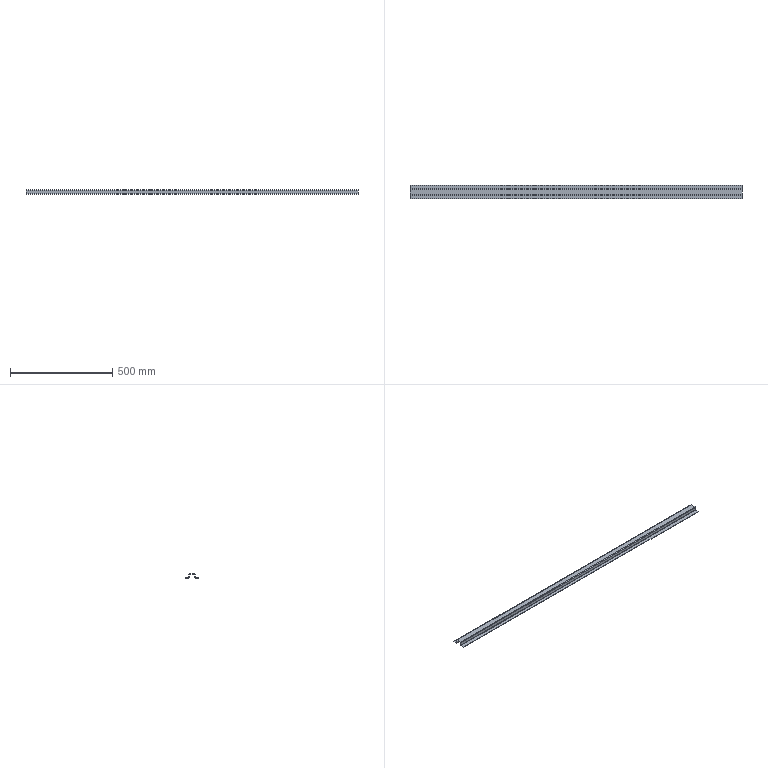Part | SolidWorks | features BaseBody 1 | 1 solid | 38 faces | box 1623 x 66 x 20 mm | volume 319907 mm3 | plane 30 | cylinder 8 | commonest cylinder face diameters 2 x4 6 x4
STEP:
#1=CARTESIAN_POINT('',(-811.4,-33.,-18.));
#2=VERTEX_POINT('',#1);
#3=CARTESIAN_POINT('',(811.4,-33.,-18.));
#4=VERTEX_POINT('',#3);
#5=CARTESIAN_POINT('',(0.,-33.,-18.));
#6=DIRECTION('',(1.,0.,0.));
#7=VECTOR('',#6,1000.);
#8=LINE('',#5,#7);
#9=EDGE_CURVE('',#2,#4,#8,.T.);
#10=ORIENTED_EDGE('',*,*,#9,.F.);
#11=CARTESIAN_POINT('',(-811.4,-33.,-20.));
#12=VERTEX_POINT('',#11);
#13=CARTESIAN_POINT('',(-811.4,-33.,-20.));
#14=DIRECTION('',(0.,0.,1.));
#15=VECTOR('',#14,1000.);
#16=LINE('',#13,#15);
#17=EDGE_CURVE('',#12,#2,#16,.T.);
#18=ORIENTED_EDGE('',*,*,#17,.F.);
#19=CARTESIAN_POINT('',(811.4,-33.,-20.));
#20=VERTEX_POINT('',#19);
#21=CARTESIAN_POINT('',(-811.4,-33.,-20.));
#22=DIRECTION('',(1.,0.,0.));
#23=VECTOR('',#22,1000.);
#24=LINE('',#21,#23);
#25=EDGE_CURVE('',#12,#20,#24,.T.);
#26=ORIENTED_EDGE('',*,*,#25,.T.);
#27=CARTESIAN_POINT('',(811.4,-33.,-20.));
#28=DIRECTION('',(0.,0.,1.));
#29=VECTOR('',#28,1000.);
#30=LINE('',#27,#29);
#31=EDGE_CURVE('',#20,#4,#30,.T.);
#32=ORIENTED_EDGE('',*,*,#31,.T.);
#33=EDGE_LOOP('',(#10,#18,#26,#32));
#34=FACE_OUTER_BOUND('',#33,.T.);
#35=CARTESIAN_POINT('',(-811.4,-33.,-20.));
#36=DIRECTION('',(0.,-1.,0.));
#37=DIRECTION('',(0.,0.,-1.));
#38=AXIS2_PLACEMENT_3D('',#35,#36,#37);
#39=PLANE('',#38);
#40=ADVANCED_FACE('',(#34),#39,.T.);
#41=CARTESIAN_POINT('',(811.4,-16.,-18.));
#42=VERTEX_POINT('',#41);
#43=CARTESIAN_POINT('',(811.4,0.,-18.));
#44=DIRECTION('',(0.,1.,0.));
#45=VECTOR('',#44,1000.);
#46=LINE('',#43,#45);
#47=EDGE_CURVE('',#4,#42,#46,.T.);
#48=ORIENTED_EDGE('',*,*,#47,.T.);
#49=CARTESIAN_POINT('',(-811.4,-16.,-18.));
#50=VERTEX_POINT('',#49);
#51=CARTESIAN_POINT('',(-811.4,-16.,-18.));
#52=DIRECTION('',(1.,0.,0.));
#53=VECTOR('',#52,1000.);
#54=LINE('',#51,#53);
#55=EDGE_CURVE('',#50,#42,#54,.T.);
#56=ORIENTED_EDGE('',*,*,#55,.F.);
#57=CARTESIAN_POINT('',(-811.4,0.,-18.));
#58=DIRECTION('',(0.,-1.,0.));
#59=VECTOR('',#58,1000.);
#60=LINE('',#57,#59);
#61=EDGE_CURVE('',#50,#2,#60,.T.);
#62=ORIENTED_EDGE('',*,*,#61,.T.);
#63=ORIENTED_EDGE('',*,*,#9,.T.);
#64=EDGE_LOOP('',(#48,#56,#62,#63));
#65=FACE_OUTER_BOUND('',#64,.T.);
#66=CARTESIAN_POINT('',(0.,0.,-18.));
#67=DIRECTION('',(0.,0.,1.));
#68=DIRECTION('',(1.,0.,0.));
#69=AXIS2_PLACEMENT_3D('',#66,#67,#68);
#70=PLANE('',#69);
#71=ADVANCED_FACE('',(#65),#70,.T.);
#72=CARTESIAN_POINT('',(811.4,-16.,-20.));
#73=VERTEX_POINT('',#72);
#74=CARTESIAN_POINT('',(-811.4,-16.,-20.));
#75=VERTEX_POINT('',#74);
#76=CARTESIAN_POINT('',(-811.4,-16.,-20.));
#77=DIRECTION('',(-1.,0.,0.));
#78=VECTOR('',#77,1000.);
#79=LINE('',#76,#78);
#80=EDGE_CURVE('',#73,#75,#79,.T.);
#81=ORIENTED_EDGE('',*,*,#80,.F.);
#82=CARTESIAN_POINT('',(811.4,-33.,-20.));
#83=DIRECTION('',(0.,1.,0.));
#84=VECTOR('',#83,1000.);
#85=LINE('',#82,#84);
#86=EDGE_CURVE('',#20,#73,#85,.T.);
#87=ORIENTED_EDGE('',*,*,#86,.F.);
#88=ORIENTED_EDGE('',*,*,#25,.F.);
#89=CARTESIAN_POINT('',(-811.4,-15.,-20.));
#90=DIRECTION('',(0.,-1.,0.));
#91=VECTOR('',#90,1000.);
#92=LINE('',#89,#91);
#93=EDGE_CURVE('',#75,#12,#92,.T.);
#94=ORIENTED_EDGE('',*,*,#93,.F.);
#95=EDGE_LOOP('',(#81,#87,#88,#94));
#96=FACE_OUTER_BOUND('',#95,.T.);
#97=CARTESIAN_POINT('',(0.,0.,-20.));
#98=DIRECTION('',(0.,0.,1.));
#99=DIRECTION('',(1.,0.,0.));
#100=AXIS2_PLACEMENT_3D('',#97,#98,#99);
#101=PLANE('',#100);
#102=ADVANCED_FACE('',(#96),#101,.F.);
#103=ORIENTED_EDGE('',*,*,#86,.T.);
#104=CARTESIAN_POINT('',(811.4,-16.,-18.));
#105=DIRECTION('',(0.,0.,-1.));
#106=VECTOR('',#105,1000.);
#107=LINE('',#104,#106);
#108=EDGE_CURVE('',#42,#73,#107,.T.);
#109=ORIENTED_EDGE('',*,*,#108,.F.);
#110=ORIENTED_EDGE('',*,*,#47,.F.);
#111=ORIENTED_EDGE('',*,*,#31,.F.);
#112=EDGE_LOOP('',(#103,#109,#110,#111));
#113=FACE_OUTER_BOUND('',#112,.T.);
#114=CARTESIAN_POINT('',(811.4,-33.,-20.));
#115=DIRECTION('',(1.,0.,0.));
#116=DIRECTION('',(0.,0.,-1.));
#117=AXIS2_PLACEMENT_3D('',#114,#115,#116);
#118=PLANE('',#117);
#119=ADVANCED_FACE('',(#113),#118,.T.);
#120=ORIENTED_EDGE('',*,*,#61,.F.);
#121=CARTESIAN_POINT('',(-811.4,-16.,-20.));
#122=DIRECTION('',(0.,0.,-1.));
#123=VECTOR('',#122,1000.);
#124=LINE('',#121,#123);
#125=EDGE_CURVE('',#50,#75,#124,.T.);
#126=ORIENTED_EDGE('',*,*,#125,.T.);
#127=ORIENTED_EDGE('',*,*,#93,.T.);
#128=ORIENTED_EDGE('',*,*,#17,.T.);
#129=EDGE_LOOP('',(#120,#126,#127,#128));
#130=FACE_OUTER_BOUND('',#129,.T.);
#131=CARTESIAN_POINT('',(-811.4,-15.,-20.));
#132=DIRECTION('',(-1.,0.,0.));
#133=DIRECTION('',(0.,1.,0.));
#134=AXIS2_PLACEMENT_3D('',#131,#132,#133);
#135=PLANE('',#134);
#136=ADVANCED_FACE('',(#130),#135,.T.);
#137=CARTESIAN_POINT('',(811.4,-15.,-17.));
#138=VERTEX_POINT('',#137);
#139=CARTESIAN_POINT('',(-811.4,-15.,-17.));
#140=VERTEX_POINT('',#139);
#141=CARTESIAN_POINT('',(811.4,-15.,-17.));
#142=DIRECTION('',(-1.,0.,0.));
#143=VECTOR('',#142,1000.);
#144=LINE('',#141,#143);
#145=EDGE_CURVE('',#138,#140,#144,.T.);
#146=ORIENTED_EDGE('',*,*,#145,.T.);
#147=CARTESIAN_POINT('',(-811.4,-16.,-17.));
#148=DIRECTION('',(-1.,0.,0.));
#149=DIRECTION('',(0.,0.,-1.));
#150=AXIS2_PLACEMENT_3D('',#147,#148,#149);
#151=CIRCLE('',#150,1.);
#152=EDGE_CURVE('',#140,#50,#151,.T.);
#153=ORIENTED_EDGE('',*,*,#152,.T.);
#154=ORIENTED_EDGE('',*,*,#55,.T.);
#155=CARTESIAN_POINT('',(811.4,-16.,-17.));
#156=DIRECTION('',(1.,0.,0.));
#157=DIRECTION('',(0.,0.,-1.));
#158=AXIS2_PLACEMENT_3D('',#155,#156,#157);
#159=CIRCLE('',#158,1.);
#160=EDGE_CURVE('',#42,#138,#159,.T.);
#161=ORIENTED_EDGE('',*,*,#160,.T.);
#162=EDGE_LOOP('',(#146,#153,#154,#161));
#163=FACE_OUTER_BOUND('',#162,.T.);
#164=CARTESIAN_POINT('',(811.4,-16.,-17.));
#165=DIRECTION('',(1.,0.,0.));
#166=DIRECTION('',(0.,0.,-1.));
#167=AXIS2_PLACEMENT_3D('',#164,#165,#166);
#168=CYLINDRICAL_SURFACE('',#167,1.);
#169=ADVANCED_FACE('',(#163),#168,.F.);
#170=CARTESIAN_POINT('',(811.4,-13.,-17.));
#171=VERTEX_POINT('',#170);
#172=CARTESIAN_POINT('',(-811.4,-13.,-17.));
#173=VERTEX_POINT('',#172);
#174=CARTESIAN_POINT('',(811.4,-13.,-17.));
#175=DIRECTION('',(-1.,0.,0.));
#176=VECTOR('',#175,1000.);
#177=LINE('',#174,#176);
#178=EDGE_CURVE('',#171,#173,#177,.T.);
#179=ORIENTED_EDGE('',*,*,#178,.F.);
#180=CARTESIAN_POINT('',(811.4,-16.,-17.));
#181=DIRECTION('',(1.,0.,0.));
#182=DIRECTION('',(0.,0.,-1.));
#183=AXIS2_PLACEMENT_3D('',#180,#181,#182);
#184=CIRCLE('',#183,3.);
#185=EDGE_CURVE('',#73,#171,#184,.T.);
#186=ORIENTED_EDGE('',*,*,#185,.F.);
#187=ORIENTED_EDGE('',*,*,#80,.T.);
#188=CARTESIAN_POINT('',(-811.4,-16.,-17.));
#189=DIRECTION('',(-1.,0.,0.));
#190=DIRECTION('',(0.,0.,-1.));
#191=AXIS2_PLACEMENT_3D('',#188,#189,#190);
#192=CIRCLE('',#191,3.);
#193=EDGE_CURVE('',#173,#75,#192,.T.);
#194=ORIENTED_EDGE('',*,*,#193,.F.);
#195=EDGE_LOOP('',(#179,#186,#187,#194));
#196=FACE_OUTER_BOUND('',#195,.T.);
#197=CARTESIAN_POINT('',(811.4,-16.,-17.));
#198=DIRECTION('',(1.,0.,0.));
#199=DIRECTION('',(0.,0.,-1.));
#200=AXIS2_PLACEMENT_3D('',#197,#198,#199);
#201=CYLINDRICAL_SURFACE('',#200,3.);
#202=ADVANCED_FACE('',(#196),#201,.T.);
#203=ORIENTED_EDGE('',*,*,#160,.F.);
#204=ORIENTED_EDGE('',*,*,#108,.T.);
#205=ORIENTED_EDGE('',*,*,#185,.T.);
#206=CARTESIAN_POINT('',(811.4,-15.,-17.));
#207=DIRECTION('',(0.,1.,0.));
#208=VECTOR('',#207,1000.);
#209=LINE('',#206,#208);
#210=EDGE_CURVE('',#138,#171,#209,.T.);
#211=ORIENTED_EDGE('',*,*,#210,.F.);
#212=EDGE_LOOP('',(#203,#204,#205,#211));
#213=FACE_OUTER_BOUND('',#212,.T.);
#214=CARTESIAN_POINT('',(811.4,-16.,-17.));
#215=DIRECTION('',(-1.,0.,0.));
#216=DIRECTION('',(0.,0.,1.));
#217=AXIS2_PLACEMENT_3D('',#214,#215,#216);
#218=PLANE('',#217);
#219=ADVANCED_FACE('',(#213),#218,.F.);
#220=ORIENTED_EDGE('',*,*,#125,.F.);
#221=ORIENTED_EDGE('',*,*,#152,.F.);
#222=CARTESIAN_POINT('',(-811.4,-15.,-17.));
#223=DIRECTION('',(0.,1.,0.));
#224=VECTOR('',#223,1000.);
#225=LINE('',#222,#224);
#226=EDGE_CURVE('',#140,#173,#225,.T.);
#227=ORIENTED_EDGE('',*,*,#226,.T.);
#228=ORIENTED_EDGE('',*,*,#193,.T.);
#229=EDGE_LOOP('',(#220,#221,#227,#228));
#230=FACE_OUTER_BOUND('',#229,.T.);
#231=CARTESIAN_POINT('',(-811.4,-16.,-17.));
#232=DIRECTION('',(-1.,0.,0.));
#233=DIRECTION('',(0.,0.,1.));
#234=AXIS2_PLACEMENT_3D('',#231,#232,#233);
#235=PLANE('',#234);
#236=ADVANCED_FACE('',(#230),#235,.T.);
#237=CARTESIAN_POINT('',(811.4,33.,-18.));
#238=VERTEX_POINT('',#237);
#239=CARTESIAN_POINT('',(-811.4,33.,-18.));
#240=VERTEX_POINT('',#239);
#241=CARTESIAN_POINT('',(0.,33.,-18.));
#242=DIRECTION('',(-1.,0.,0.));
#243=VECTOR('',#242,1000.);
#244=LINE('',#241,#243);
#245=EDGE_CURVE('',#238,#240,#244,.T.);
#246=ORIENTED_EDGE('',*,*,#245,.F.);
#247=CARTESIAN_POINT('',(811.4,33.,-20.));
#248=VERTEX_POINT('',#247);
#249=CARTESIAN_POINT('',(811.4,33.,-20.));
#250=DIRECTION('',(0.,0.,1.));
#251=VECTOR('',#250,1000.);
#252=LINE('',#249,#251);
#253=EDGE_CURVE('',#248,#238,#252,.T.);
#254=ORIENTED_EDGE('',*,*,#253,.F.);
#255=CARTESIAN_POINT('',(-811.4,33.,-20.));
#256=VERTEX_POINT('',#255);
#257=CARTESIAN_POINT('',(-811.4,33.,-20.));
#258=DIRECTION('',(-1.,0.,0.));
#259=VECTOR('',#258,1000.);
#260=LINE('',#257,#259);
#261=EDGE_CURVE('',#248,#256,#260,.T.);
#262=ORIENTED_EDGE('',*,*,#261,.T.);
#263=CARTESIAN_POINT('',(-811.4,33.,-20.));
#264=DIRECTION('',(0.,0.,1.));
#265=VECTOR('',#264,1000.);
#266=LINE('',#263,#265);
#267=EDGE_CURVE('',#256,#240,#266,.T.);
#268=ORIENTED_EDGE('',*,*,#267,.T.);
#269=EDGE_LOOP('',(#246,#254,#262,#268));
#270=FACE_OUTER_BOUND('',#269,.T.);
#271=CARTESIAN_POINT('',(-811.4,33.,-20.));
#272=DIRECTION('',(0.,1.,0.));
#273=DIRECTION('',(1.,0.,0.));
#274=AXIS2_PLACEMENT_3D('',#271,#272,#273);
#275=PLANE('',#274);
#276=ADVANCED_FACE('',(#270),#275,.T.);
#277=CARTESIAN_POINT('',(811.4,16.,-18.));
#278=VERTEX_POINT('',#277);
#279=CARTESIAN_POINT('',(-811.4,16.,-18.));
#280=VERTEX_POINT('',#279);
#281=CARTESIAN_POINT('',(811.4,16.,-18.));
#282=DIRECTION('',(-1.,0.,0.));
#283=VECTOR('',#282,1000.);
#284=LINE('',#281,#283);
#285=EDGE_CURVE('',#278,#280,#284,.T.);
#286=ORIENTED_EDGE('',*,*,#285,.F.);
#287=CARTESIAN_POINT('',(811.4,0.,-18.));
#288=DIRECTION('',(0.,1.,0.));
#289=VECTOR('',#288,1000.);
#290=LINE('',#287,#289);
#291=EDGE_CURVE('',#278,#238,#290,.T.);
#292=ORIENTED_EDGE('',*,*,#291,.T.);
#293=ORIENTED_EDGE('',*,*,#245,.T.);
#294=CARTESIAN_POINT('',(-811.4,0.,-18.));
#295=DIRECTION('',(0.,-1.,0.));
#296=VECTOR('',#295,1000.);
#297=LINE('',#294,#296);
#298=EDGE_CURVE('',#240,#280,#297,.T.);
#299=ORIENTED_EDGE('',*,*,#298,.T.);
#300=EDGE_LOOP('',(#286,#292,#293,#299));
#301=FACE_OUTER_BOUND('',#300,.T.);
#302=CARTESIAN_POINT('',(0.,0.,-18.));
#303=DIRECTION('',(0.,0.,-1.));
#304=DIRECTION('',(0.,-1.,0.));
#305=AXIS2_PLACEMENT_3D('',#302,#303,#304);
#306=PLANE('',#305);
#307=ADVANCED_FACE('',(#301),#306,.F.);
#308=CARTESIAN_POINT('',(811.4,16.,-20.));
#309=VERTEX_POINT('',#308);
#310=CARTESIAN_POINT('',(811.4,33.,-20.));
#311=DIRECTION('',(0.,1.,0.));
#312=VECTOR('',#311,1000.);
#313=LINE('',#310,#312);
#314=EDGE_CURVE('',#309,#248,#313,.T.);
#315=ORIENTED_EDGE('',*,*,#314,.F.);
#316=CARTESIAN_POINT('',(-811.4,16.,-20.));
#317=VERTEX_POINT('',#316);
#318=CARTESIAN_POINT('',(0.,16.,-20.));
#319=DIRECTION('',(-1.,0.,0.));
#320=VECTOR('',#319,1000.);
#321=LINE('',#318,#320);
#322=EDGE_CURVE('',#309,#317,#321,.T.);
#323=ORIENTED_EDGE('',*,*,#322,.T.);
#324=CARTESIAN_POINT('',(-811.4,33.,-20.));
#325=DIRECTION('',(0.,-1.,0.));
#326=VECTOR('',#325,1000.);
#327=LINE('',#324,#326);
#328=EDGE_CURVE('',#256,#317,#327,.T.);
#329=ORIENTED_EDGE('',*,*,#328,.F.);
#330=ORIENTED_EDGE('',*,*,#261,.F.);
#331=EDGE_LOOP('',(#315,#323,#329,#330));
#332=FACE_OUTER_BOUND('',#331,.T.);
#333=CARTESIAN_POINT('',(0.,0.,-20.));
#334=DIRECTION('',(0.,0.,-1.));
#335=DIRECTION('',(0.,-1.,0.));
#336=AXIS2_PLACEMENT_3D('',#333,#334,#335);
#337=PLANE('',#336);
#338=ADVANCED_FACE('',(#332),#337,.T.);
#339=ORIENTED_EDGE('',*,*,#328,.T.);
#340=CARTESIAN_POINT('',(-811.4,16.,-18.));
#341=DIRECTION('',(0.,0.,-1.));
#342=VECTOR('',#341,1000.);
#343=LINE('',#340,#342);
#344=EDGE_CURVE('',#280,#317,#343,.T.);
#345=ORIENTED_EDGE('',*,*,#344,.F.);
#346=ORIENTED_EDGE('',*,*,#298,.F.);
#347=ORIENTED_EDGE('',*,*,#267,.F.);
#348=EDGE_LOOP('',(#339,#345,#346,#347));
#349=FACE_OUTER_BOUND('',#348,.T.);
#350=CARTESIAN_POINT('',(-811.4,33.,-20.));
#351=DIRECTION('',(-1.,0.,0.));
#352=DIRECTION('',(0.,0.,1.));
#353=AXIS2_PLACEMENT_3D('',#350,#351,#352);
#354=PLANE('',#353);
#355=ADVANCED_FACE('',(#349),#354,.T.);
#356=ORIENTED_EDGE('',*,*,#291,.F.);
#357=CARTESIAN_POINT('',(811.4,16.,-20.));
#358=DIRECTION('',(0.,0.,-1.));
#359=VECTOR('',#358,1000.);
#360=LINE('',#357,#359);
#361=EDGE_CURVE('',#278,#309,#360,.T.);
#362=ORIENTED_EDGE('',*,*,#361,.T.);
#363=ORIENTED_EDGE('',*,*,#314,.T.);
#364=ORIENTED_EDGE('',*,*,#253,.T.);
#365=EDGE_LOOP('',(#356,#362,#363,#364));
#366=FACE_OUTER_BOUND('',#365,.T.);
#367=CARTESIAN_POINT('',(811.4,33.,-20.));
#368=DIRECTION('',(1.,0.,0.));
#369=DIRECTION('',(0.,1.,0.));
#370=AXIS2_PLACEMENT_3D('',#367,#368,#369);
#371=PLANE('',#370);
#372=ADVANCED_FACE('',(#366),#371,.T.);
#373=CARTESIAN_POINT('',(-811.4,15.,-17.));
#374=VERTEX_POINT('',#373);
#375=CARTESIAN_POINT('',(811.4,15.,-17.));
#376=VERTEX_POINT('',#375);
#377=CARTESIAN_POINT('',(-811.4,15.,-17.));
#378=DIRECTION('',(1.,0.,0.));
#379=VECTOR('',#378,1000.);
#380=LINE('',#377,#379);
#381=EDGE_CURVE('',#374,#376,#380,.T.);
#382=ORIENTED_EDGE('',*,*,#381,.T.);
#383=CARTESIAN_POINT('',(811.4,16.,-17.));
#384=DIRECTION('',(1.,0.,0.));
#385=DIRECTION('',(0.,0.,1.));
#386=AXIS2_PLACEMENT_3D('',#383,#384,#385);
#387=CIRCLE('',#386,1.);
#388=EDGE_CURVE('',#376,#278,#387,.T.);
#389=ORIENTED_EDGE('',*,*,#388,.T.);
#390=ORIENTED_EDGE('',*,*,#285,.T.);
#391=CARTESIAN_POINT('',(-811.4,16.,-17.));
#392=DIRECTION('',(-1.,0.,0.));
#393=DIRECTION('',(0.,0.,1.));
#394=AXIS2_PLACEMENT_3D('',#391,#392,#393);
#395=CIRCLE('',#394,1.);
#396=EDGE_CURVE('',#280,#374,#395,.T.);
#397=ORIENTED_EDGE('',*,*,#396,.T.);
#398=EDGE_LOOP('',(#382,#389,#390,#397));
#399=FACE_OUTER_BOUND('',#398,.T.);
#400=CARTESIAN_POINT('',(-811.4,16.,-17.));
#401=DIRECTION('',(-1.,0.,0.));
#402=DIRECTION('',(0.,0.,-1.));
#403=AXIS2_PLACEMENT_3D('',#400,#401,#402);
#404=CYLINDRICAL_SURFACE('',#403,1.);
#405=ADVANCED_FACE('',(#399),#404,.F.);
#406=CARTESIAN_POINT('',(-811.4,13.,-17.));
#407=VERTEX_POINT('',#406);
#408=CARTESIAN_POINT('',(811.4,13.,-17.));
#409=VERTEX_POINT('',#408);
#410=CARTESIAN_POINT('',(-811.4,13.,-17.));
#411=DIRECTION('',(1.,0.,0.));
#412=VECTOR('',#411,1000.);
#413=LINE('',#410,#412);
#414=EDGE_CURVE('',#407,#409,#413,.T.);
#415=ORIENTED_EDGE('',*,*,#414,.F.);
#416=CARTESIAN_POINT('',(-811.4,16.,-17.));
#417=DIRECTION('',(-1.,0.,0.));
#418=DIRECTION('',(0.,0.,1.));
#419=AXIS2_PLACEMENT_3D('',#416,#417,#418);
#420=CIRCLE('',#419,3.);
#421=EDGE_CURVE('',#317,#407,#420,.T.);
#422=ORIENTED_EDGE('',*,*,#421,.F.);
#423=ORIENTED_EDGE('',*,*,#322,.F.);
#424=CARTESIAN_POINT('',(811.4,16.,-17.));
#425=DIRECTION('',(1.,0.,0.));
#426=DIRECTION('',(0.,0.,1.));
#427=AXIS2_PLACEMENT_3D('',#424,#425,#426);
#428=CIRCLE('',#427,3.);
#429=EDGE_CURVE('',#409,#309,#428,.T.);
#430=ORIENTED_EDGE('',*,*,#429,.F.);
#431=EDGE_LOOP('',(#415,#422,#423,#430));
#432=FACE_OUTER_BOUND('',#431,.T.);
#433=CARTESIAN_POINT('',(-811.4,16.,-17.));
#434=DIRECTION('',(-1.,0.,0.));
#435=DIRECTION('',(0.,0.,-1.));
#436=AXIS2_PLACEMENT_3D('',#433,#434,#435);
#437=CYLINDRICAL_SURFACE('',#436,3.);
#438=ADVANCED_FACE('',(#432),#437,.T.);
#439=ORIENTED_EDGE('',*,*,#396,.F.);
#440=ORIENTED_EDGE('',*,*,#344,.T.);
#441=ORIENTED_EDGE('',*,*,#421,.T.);
#442=CARTESIAN_POINT('',(-811.4,15.,-17.));
#443=DIRECTION('',(0.,-1.,0.));
#444=VECTOR('',#443,1000.);
#445=LINE('',#442,#444);
#446=EDGE_CURVE('',#374,#407,#445,.T.);
#447=ORIENTED_EDGE('',*,*,#446,.F.);
#448=EDGE_LOOP('',(#439,#440,#441,#447));
#449=FACE_OUTER_BOUND('',#448,.T.);
#450=CARTESIAN_POINT('',(-811.4,16.,-17.));
#451=DIRECTION('',(1.,0.,0.));
#452=DIRECTION('',(0.,1.,0.));
#453=AXIS2_PLACEMENT_3D('',#450,#451,#452);
#454=PLANE('',#453);
#455=ADVANCED_FACE('',(#449),#454,.F.);
#456=ORIENTED_EDGE('',*,*,#361,.F.);
#457=ORIENTED_EDGE('',*,*,#388,.F.);
#458=CARTESIAN_POINT('',(811.4,15.,-17.));
#459=DIRECTION('',(0.,-1.,0.));
#460=VECTOR('',#459,1000.);
#461=LINE('',#458,#460);
#462=EDGE_CURVE('',#376,#409,#461,.T.);
#463=ORIENTED_EDGE('',*,*,#462,.T.);
#464=ORIENTED_EDGE('',*,*,#429,.T.);
#465=EDGE_LOOP('',(#456,#457,#463,#464));
#466=FACE_OUTER_BOUND('',#465,.T.);
#467=CARTESIAN_POINT('',(811.4,16.,-17.));
#468=DIRECTION('',(1.,0.,0.));
#469=DIRECTION('',(0.,1.,0.));
#470=AXIS2_PLACEMENT_3D('',#467,#468,#469);
#471=PLANE('',#470);
#472=ADVANCED_FACE('',(#466),#471,.T.);
#473=ORIENTED_EDGE('',*,*,#226,.F.);
#474=CARTESIAN_POINT('',(-811.4,-15.,-3.));
#475=VERTEX_POINT('',#474);
#476=CARTESIAN_POINT('',(-811.4,-15.,-20.));
#477=DIRECTION('',(0.,0.,1.));
#478=VECTOR('',#477,1000.);
#479=LINE('',#476,#478);
#480=EDGE_CURVE('',#140,#475,#479,.T.);
#481=ORIENTED_EDGE('',*,*,#480,.T.);
#482=CARTESIAN_POINT('',(-811.4,-13.,-3.));
#483=VERTEX_POINT('',#482);
#484=CARTESIAN_POINT('',(-811.4,-13.,-3.));
#485=DIRECTION('',(0.,-1.,0.));
#486=VECTOR('',#485,1000.);
#487=LINE('',#484,#486);
#488=EDGE_CURVE('',#483,#475,#487,.T.);
#489=ORIENTED_EDGE('',*,*,#488,.F.);
#490=CARTESIAN_POINT('',(-811.4,-13.,0.));
#491=DIRECTION('',(0.,0.,1.));
#492=VECTOR('',#491,1000.);
#493=LINE('',#490,#492);
#494=EDGE_CURVE('',#173,#483,#493,.T.);
#495=ORIENTED_EDGE('',*,*,#494,.F.);
#496=EDGE_LOOP('',(#473,#481,#489,#495));
#497=FACE_OUTER_BOUND('',#496,.T.);
#498=CARTESIAN_POINT('',(-811.4,-15.,-20.));
#499=DIRECTION('',(-1.,0.,0.));
#500=DIRECTION('',(0.,0.,1.));
#501=AXIS2_PLACEMENT_3D('',#498,#499,#500);
#502=PLANE('',#501);
#503=ADVANCED_FACE('',(#497),#502,.T.);
#504=CARTESIAN_POINT('',(-811.4,-12.,-2.));
#505=VERTEX_POINT('',#504);
#506=CARTESIAN_POINT('',(811.4,-12.,-2.));
#507=VERTEX_POINT('',#506);
#508=CARTESIAN_POINT('',(-811.4,-12.,-2.));
#509=DIRECTION('',(1.,0.,0.));
#510=VECTOR('',#509,1000.);
#511=LINE('',#508,#510);
#512=EDGE_CURVE('',#505,#507,#511,.T.);
#513=ORIENTED_EDGE('',*,*,#512,.T.);
#514=CARTESIAN_POINT('',(811.4,-13.,-3.));
#515=VERTEX_POINT('',#514);
#516=CARTESIAN_POINT('',(811.4,-12.,-3.));
#517=DIRECTION('',(1.,0.,0.));
#518=DIRECTION('',(0.,0.,1.));
#519=AXIS2_PLACEMENT_3D('',#516,#517,#518);
#520=CIRCLE('',#519,1.);
#521=EDGE_CURVE('',#507,#515,#520,.T.);
#522=ORIENTED_EDGE('',*,*,#521,.T.);
#523=CARTESIAN_POINT('',(811.4,-13.,-3.));
#524=DIRECTION('',(-1.,0.,0.));
#525=VECTOR('',#524,1000.);
#526=LINE('',#523,#525);
#527=EDGE_CURVE('',#515,#483,#526,.T.);
#528=ORIENTED_EDGE('',*,*,#527,.T.);
#529=CARTESIAN_POINT('',(-811.4,-12.,-3.));
#530=DIRECTION('',(-1.,0.,0.));
#531=DIRECTION('',(0.,0.,1.));
#532=AXIS2_PLACEMENT_3D('',#529,#530,#531);
#533=CIRCLE('',#532,1.);
#534=EDGE_CURVE('',#483,#505,#533,.T.);
#535=ORIENTED_EDGE('',*,*,#534,.T.);
#536=EDGE_LOOP('',(#513,#522,#528,#535));
#537=FACE_OUTER_BOUND('',#536,.T.);
#538=CARTESIAN_POINT('',(-811.4,-12.,-3.));
#539=DIRECTION('',(-1.,0.,0.));
#540=DIRECTION('',(0.,-1.,0.));
#541=AXIS2_PLACEMENT_3D('',#538,#539,#540);
#542=CYLINDRICAL_SURFACE('',#541,1.);
#543=ADVANCED_FACE('',(#537),#542,.F.);
#544=CARTESIAN_POINT('',(-811.4,-12.,0.));
#545=VERTEX_POINT('',#544);
#546=CARTESIAN_POINT('',(811.4,-12.,0.));
#547=VERTEX_POINT('',#546);
#548=CARTESIAN_POINT('',(-811.4,-12.,0.));
#549=DIRECTION('',(1.,0.,0.));
#550=VECTOR('',#549,1000.);
#551=LINE('',#548,#550);
#552=EDGE_CURVE('',#545,#547,#551,.T.);
#553=ORIENTED_EDGE('',*,*,#552,.F.);
#554=CARTESIAN_POINT('',(-811.4,-12.,-3.));
#555=DIRECTION('',(-1.,0.,0.));
#556=DIRECTION('',(0.,0.,1.));
#557=AXIS2_PLACEMENT_3D('',#554,#555,#556);
#558=CIRCLE('',#557,3.);
#559=EDGE_CURVE('',#475,#545,#558,.T.);
#560=ORIENTED_EDGE('',*,*,#559,.F.);
#561=CARTESIAN_POINT('',(811.4,-15.,-3.));
#562=VERTEX_POINT('',#561);
#563=CARTESIAN_POINT('',(811.4,-15.,-3.));
#564=DIRECTION('',(1.,0.,0.));
#565=VECTOR('',#564,1000.);
#566=LINE('',#563,#565);
#567=EDGE_CURVE('',#475,#562,#566,.T.);
#568=ORIENTED_EDGE('',*,*,#567,.T.);
#569=CARTESIAN_POINT('',(811.4,-12.,-3.));
#570=DIRECTION('',(1.,0.,0.));
#571=DIRECTION('',(0.,0.,1.));
#572=AXIS2_PLACEMENT_3D('',#569,#570,#571);
#573=CIRCLE('',#572,3.);
#574=EDGE_CURVE('',#547,#562,#573,.T.);
#575=ORIENTED_EDGE('',*,*,#574,.F.);
#576=EDGE_LOOP('',(#553,#560,#568,#575));
#577=FACE_OUTER_BOUND('',#576,.T.);
#578=CARTESIAN_POINT('',(-811.4,-12.,-3.));
#579=DIRECTION('',(-1.,0.,0.));
#580=DIRECTION('',(0.,-1.,0.));
#581=AXIS2_PLACEMENT_3D('',#578,#579,#580);
#582=CYLINDRICAL_SURFACE('',#581,3.);
#583=ADVANCED_FACE('',(#577),#582,.T.);
#584=ORIENTED_EDGE('',*,*,#534,.F.);
#585=ORIENTED_EDGE('',*,*,#488,.T.);
#586=ORIENTED_EDGE('',*,*,#559,.T.);
#587=CARTESIAN_POINT('',(-811.4,-12.,-2.));
#588=DIRECTION('',(0.,0.,1.));
#589=VECTOR('',#588,1000.);
#590=LINE('',#587,#589);
#591=EDGE_CURVE('',#505,#545,#590,.T.);
#592=ORIENTED_EDGE('',*,*,#591,.F.);
#593=EDGE_LOOP('',(#584,#585,#586,#592));
#594=FACE_OUTER_BOUND('',#593,.T.);
#595=CARTESIAN_POINT('',(-811.4,-12.,-3.));
#596=DIRECTION('',(1.,0.,0.));
#597=DIRECTION('',(0.,1.,0.));
#598=AXIS2_PLACEMENT_3D('',#595,#596,#597);
#599=PLANE('',#598);
#600=ADVANCED_FACE('',(#594),#599,.F.);
#601=CARTESIAN_POINT('',(811.4,-15.,-3.));
#602=DIRECTION('',(0.,-1.,0.));
#603=VECTOR('',#602,1000.);
#604=LINE('',#601,#603);
#605=EDGE_CURVE('',#515,#562,#604,.T.);
#606=ORIENTED_EDGE('',*,*,#605,.F.);
#607=ORIENTED_EDGE('',*,*,#521,.F.);
#608=CARTESIAN_POINT('',(811.4,-12.,-2.));
#609=DIRECTION('',(0.,0.,1.));
#610=VECTOR('',#609,1000.);
#611=LINE('',#608,#610);
#612=EDGE_CURVE('',#507,#547,#611,.T.);
#613=ORIENTED_EDGE('',*,*,#612,.T.);
#614=ORIENTED_EDGE('',*,*,#574,.T.);
#615=EDGE_LOOP('',(#606,#607,#613,#614));
#616=FACE_OUTER_BOUND('',#615,.T.);
#617=CARTESIAN_POINT('',(811.4,-12.,-3.));
#618=DIRECTION('',(1.,0.,0.));
#619=DIRECTION('',(0.,1.,0.));
#620=AXIS2_PLACEMENT_3D('',#617,#618,#619);
#621=PLANE('',#620);
#622=ADVANCED_FACE('',(#616),#621,.T.);
#623=ORIENTED_EDGE('',*,*,#462,.F.);
#624=CARTESIAN_POINT('',(811.4,15.,-3.));
#625=VERTEX_POINT('',#624);
#626=CARTESIAN_POINT('',(811.4,15.,-2.));
#627=DIRECTION('',(0.,0.,1.));
#628=VECTOR('',#627,1000.);
#629=LINE('',#626,#628);
#630=EDGE_CURVE('',#376,#625,#629,.T.);
#631=ORIENTED_EDGE('',*,*,#630,.T.);
#632=CARTESIAN_POINT('',(811.4,13.,-3.));
#633=VERTEX_POINT('',#632);
#634=CARTESIAN_POINT('',(811.4,13.,-3.));
#635=DIRECTION('',(0.,1.,0.));
#636=VECTOR('',#635,1000.);
#637=LINE('',#634,#636);
#638=EDGE_CURVE('',#633,#625,#637,.T.);
#639=ORIENTED_EDGE('',*,*,#638,.F.);
#640=CARTESIAN_POINT('',(811.4,13.,0.));
#641=DIRECTION('',(0.,0.,1.));
#642=VECTOR('',#641,1000.);
#643=LINE('',#640,#642);
#644=EDGE_CURVE('',#409,#633,#643,.T.);
#645=ORIENTED_EDGE('',*,*,#644,.F.);
#646=EDGE_LOOP('',(#623,#631,#639,#645));
#647=FACE_OUTER_BOUND('',#646,.T.);
#648=CARTESIAN_POINT('',(811.4,15.,-2.));
#649=DIRECTION('',(1.,0.,0.));
#650=DIRECTION('',(0.,1.,0.));
#651=AXIS2_PLACEMENT_3D('',#648,#649,#650);
#652=PLANE('',#651);
#653=ADVANCED_FACE('',(#647),#652,.T.);
#654=CARTESIAN_POINT('',(811.4,12.,-2.));
#655=VERTEX_POINT('',#654);
#656=CARTESIAN_POINT('',(-811.4,12.,-2.));
#657=VERTEX_POINT('',#656);
#658=CARTESIAN_POINT('',(811.4,12.,-2.));
#659=DIRECTION('',(-1.,0.,0.));
#660=VECTOR('',#659,1000.);
#661=LINE('',#658,#660);
#662=EDGE_CURVE('',#655,#657,#661,.T.);
#663=ORIENTED_EDGE('',*,*,#662,.T.);
#664=CARTESIAN_POINT('',(-811.4,13.,-3.));
#665=VERTEX_POINT('',#664);
#666=CARTESIAN_POINT('',(-811.4,12.,-3.));
#667=DIRECTION('',(-1.,0.,0.));
#668=DIRECTION('',(0.,0.,-1.));
#669=AXIS2_PLACEMENT_3D('',#666,#667,#668);
#670=CIRCLE('',#669,1.);
#671=EDGE_CURVE('',#657,#665,#670,.T.);
#672=ORIENTED_EDGE('',*,*,#671,.T.);
#673=CARTESIAN_POINT('',(-811.4,13.,-3.));
#674=DIRECTION('',(1.,0.,0.));
#675=VECTOR('',#674,1000.);
#676=LINE('',#673,#675);
#677=EDGE_CURVE('',#665,#633,#676,.T.);
#678=ORIENTED_EDGE('',*,*,#677,.T.);
#679=CARTESIAN_POINT('',(811.4,12.,-3.));
#680=DIRECTION('',(1.,0.,0.));
#681=DIRECTION('',(0.,0.,-1.));
#682=AXIS2_PLACEMENT_3D('',#679,#680,#681);
#683=CIRCLE('',#682,1.);
#684=EDGE_CURVE('',#633,#655,#683,.T.);
#685=ORIENTED_EDGE('',*,*,#684,.T.);
#686=EDGE_LOOP('',(#663,#672,#678,#685));
#687=FACE_OUTER_BOUND('',#686,.T.);
#688=CARTESIAN_POINT('',(811.4,12.,-3.));
#689=DIRECTION('',(1.,0.,0.));
#690=DIRECTION('',(0.,1.,0.));
#691=AXIS2_PLACEMENT_3D('',#688,#689,#690);
#692=CYLINDRICAL_SURFACE('',#691,1.);
#693=ADVANCED_FACE('',(#687),#692,.F.);
#694=CARTESIAN_POINT('',(811.4,12.,0.));
#695=VERTEX_POINT('',#694);
#696=CARTESIAN_POINT('',(-811.4,12.,0.));
#697=VERTEX_POINT('',#696);
#698=CARTESIAN_POINT('',(811.4,12.,0.));
#699=DIRECTION('',(-1.,0.,0.));
#700=VECTOR('',#699,1000.);
#701=LINE('',#698,#700);
#702=EDGE_CURVE('',#695,#697,#701,.T.);
#703=ORIENTED_EDGE('',*,*,#702,.F.);
#704=CARTESIAN_POINT('',(811.4,12.,-3.));
#705=DIRECTION('',(1.,0.,0.));
#706=DIRECTION('',(0.,0.,-1.));
#707=AXIS2_PLACEMENT_3D('',#704,#705,#706);
#708=CIRCLE('',#707,3.);
#709=EDGE_CURVE('',#625,#695,#708,.T.);
#710=ORIENTED_EDGE('',*,*,#709,.F.);
#711=CARTESIAN_POINT('',(-811.4,15.,-3.));
#712=VERTEX_POINT('',#711);
#713=CARTESIAN_POINT('',(0.,15.,-3.));
#714=DIRECTION('',(1.,0.,0.));
#715=VECTOR('',#714,1000.);
#716=LINE('',#713,#715);
#717=EDGE_CURVE('',#712,#625,#716,.T.);
#718=ORIENTED_EDGE('',*,*,#717,.F.);
#719=CARTESIAN_POINT('',(-811.4,12.,-3.));
#720=DIRECTION('',(-1.,0.,0.));
#721=DIRECTION('',(0.,0.,-1.));
#722=AXIS2_PLACEMENT_3D('',#719,#720,#721);
#723=CIRCLE('',#722,3.);
#724=EDGE_CURVE('',#697,#712,#723,.T.);
#725=ORIENTED_EDGE('',*,*,#724,.F.);
#726=EDGE_LOOP('',(#703,#710,#718,#725));
#727=FACE_OUTER_BOUND('',#726,.T.);
#728=CARTESIAN_POINT('',(811.4,12.,-3.));
#729=DIRECTION('',(1.,0.,0.));
#730=DIRECTION('',(0.,1.,0.));
#731=AXIS2_PLACEMENT_3D('',#728,#729,#730);
#732=CYLINDRICAL_SURFACE('',#731,3.);
#733=ADVANCED_FACE('',(#727),#732,.T.);
#734=ORIENTED_EDGE('',*,*,#684,.F.);
#735=ORIENTED_EDGE('',*,*,#638,.T.);
#736=ORIENTED_EDGE('',*,*,#709,.T.);
#737=CARTESIAN_POINT('',(811.4,12.,-2.));
#738=DIRECTION('',(0.,0.,1.));
#739=VECTOR('',#738,1000.);
#740=LINE('',#737,#739);
#741=EDGE_CURVE('',#655,#695,#740,.T.);
#742=ORIENTED_EDGE('',*,*,#741,.F.);
#743=EDGE_LOOP('',(#734,#735,#736,#742));
#744=FACE_OUTER_BOUND('',#743,.T.);
#745=CARTESIAN_POINT('',(811.4,12.,-3.));
#746=DIRECTION('',(-1.,0.,0.));
#747=DIRECTION('',(0.,0.,1.));
#748=AXIS2_PLACEMENT_3D('',#745,#746,#747);
#749=PLANE('',#748);
#750=ADVANCED_FACE('',(#744),#749,.F.);
#751=CARTESIAN_POINT('',(-811.4,15.,-3.));
#752=DIRECTION('',(0.,1.,0.));
#753=VECTOR('',#752,1000.);
#754=LINE('',#751,#753);
#755=EDGE_CURVE('',#665,#712,#754,.T.);
#756=ORIENTED_EDGE('',*,*,#755,.F.);
#757=ORIENTED_EDGE('',*,*,#671,.F.);
#758=CARTESIAN_POINT('',(-811.4,12.,-2.));
#759=DIRECTION('',(0.,0.,1.));
#760=VECTOR('',#759,1000.);
#761=LINE('',#758,#760);
#762=EDGE_CURVE('',#657,#697,#761,.T.);
#763=ORIENTED_EDGE('',*,*,#762,.T.);
#764=ORIENTED_EDGE('',*,*,#724,.T.);
#765=EDGE_LOOP('',(#756,#757,#763,#764));
#766=FACE_OUTER_BOUND('',#765,.T.);
#767=CARTESIAN_POINT('',(-811.4,12.,-3.));
#768=DIRECTION('',(-1.,0.,0.));
#769=DIRECTION('',(0.,0.,1.));
#770=AXIS2_PLACEMENT_3D('',#767,#768,#769);
#771=PLANE('',#770);
#772=ADVANCED_FACE('',(#766),#771,.T.);
#773=ORIENTED_EDGE('',*,*,#612,.F.);
#774=CARTESIAN_POINT('',(811.4,15.,-2.));
#775=DIRECTION('',(0.,1.,0.));
#776=VECTOR('',#775,1000.);
#777=LINE('',#774,#776);
#778=EDGE_CURVE('',#507,#655,#777,.T.);
#779=ORIENTED_EDGE('',*,*,#778,.T.);
#780=ORIENTED_EDGE('',*,*,#741,.T.);
#781=CARTESIAN_POINT('',(811.4,15.,0.));
#782=DIRECTION('',(0.,1.,0.));
#783=VECTOR('',#782,1000.);
#784=LINE('',#781,#783);
#785=EDGE_CURVE('',#547,#695,#784,.T.);
#786=ORIENTED_EDGE('',*,*,#785,.F.);
#787=EDGE_LOOP('',(#773,#779,#780,#786));
#788=FACE_OUTER_BOUND('',#787,.T.);
#789=CARTESIAN_POINT('',(811.4,15.,-2.));
#790=DIRECTION('',(1.,0.,0.));
#791=DIRECTION('',(0.,1.,0.));
#792=AXIS2_PLACEMENT_3D('',#789,#790,#791);
#793=PLANE('',#792);
#794=ADVANCED_FACE('',(#788),#793,.T.);
#795=CARTESIAN_POINT('',(-811.4,15.,-2.));
#796=DIRECTION('',(0.,-1.,0.));
#797=VECTOR('',#796,1000.);
#798=LINE('',#795,#797);
#799=EDGE_CURVE('',#657,#505,#798,.T.);
#800=ORIENTED_EDGE('',*,*,#799,.T.);
#801=ORIENTED_EDGE('',*,*,#591,.T.);
#802=CARTESIAN_POINT('',(-811.4,15.,0.));
#803=DIRECTION('',(0.,-1.,0.));
#804=VECTOR('',#803,1000.);
#805=LINE('',#802,#804);
#806=EDGE_CURVE('',#697,#545,#805,.T.);
#807=ORIENTED_EDGE('',*,*,#806,.F.);
#808=ORIENTED_EDGE('',*,*,#762,.F.);
#809=EDGE_LOOP('',(#800,#801,#807,#808));
#810=FACE_OUTER_BOUND('',#809,.T.);
#811=CARTESIAN_POINT('',(-811.4,15.,-2.));
#812=DIRECTION('',(-1.,0.,0.));
#813=DIRECTION('',(0.,0.,1.));
#814=AXIS2_PLACEMENT_3D('',#811,#812,#813);
#815=PLANE('',#814);
#816=ADVANCED_FACE('',(#810),#815,.T.);
#817=ORIENTED_EDGE('',*,*,#806,.T.);
#818=ORIENTED_EDGE('',*,*,#552,.T.);
#819=ORIENTED_EDGE('',*,*,#785,.T.);
#820=ORIENTED_EDGE('',*,*,#702,.T.);
#821=EDGE_LOOP('',(#817,#818,#819,#820));
#822=FACE_OUTER_BOUND('',#821,.T.);
#823=CARTESIAN_POINT('',(0.,0.,0.));
#824=DIRECTION('',(0.,0.,1.));
#825=DIRECTION('',(1.,0.,0.));
#826=AXIS2_PLACEMENT_3D('',#823,#824,#825);
#827=PLANE('',#826);
#828=ADVANCED_FACE('',(#822),#827,.T.);
#829=ORIENTED_EDGE('',*,*,#512,.F.);
#830=ORIENTED_EDGE('',*,*,#799,.F.);
#831=ORIENTED_EDGE('',*,*,#662,.F.);
#832=ORIENTED_EDGE('',*,*,#778,.F.);
#833=EDGE_LOOP('',(#829,#830,#831,#832));
#834=FACE_OUTER_BOUND('',#833,.T.);
#835=CARTESIAN_POINT('',(0.,0.,-2.));
#836=DIRECTION('',(0.,0.,1.));
#837=DIRECTION('',(1.,0.,0.));
#838=AXIS2_PLACEMENT_3D('',#835,#836,#837);
#839=PLANE('',#838);
#840=ADVANCED_FACE('',(#834),#839,.F.);
#841=ORIENTED_EDGE('',*,*,#414,.T.);
#842=ORIENTED_EDGE('',*,*,#644,.T.);
#843=ORIENTED_EDGE('',*,*,#677,.F.);
#844=CARTESIAN_POINT('',(-811.4,13.,0.));
#845=DIRECTION('',(0.,0.,-1.));
#846=VECTOR('',#845,1000.);
#847=LINE('',#844,#846);
#848=EDGE_CURVE('',#665,#407,#847,.T.);
#849=ORIENTED_EDGE('',*,*,#848,.T.);
#850=EDGE_LOOP('',(#841,#842,#843,#849));
#851=FACE_OUTER_BOUND('',#850,.T.);
#852=CARTESIAN_POINT('',(0.,13.,0.));
#853=DIRECTION('',(0.,1.,0.));
#854=DIRECTION('',(0.,0.,-1.));
#855=AXIS2_PLACEMENT_3D('',#852,#853,#854);
#856=PLANE('',#855);
#857=ADVANCED_FACE('',(#851),#856,.F.);
#858=ORIENTED_EDGE('',*,*,#630,.F.);
#859=ORIENTED_EDGE('',*,*,#381,.F.);
#860=CARTESIAN_POINT('',(-811.4,15.,-20.));
#861=DIRECTION('',(0.,0.,-1.));
#862=VECTOR('',#861,1000.);
#863=LINE('',#860,#862);
#864=EDGE_CURVE('',#712,#374,#863,.T.);
#865=ORIENTED_EDGE('',*,*,#864,.F.);
#866=ORIENTED_EDGE('',*,*,#717,.T.);
#867=EDGE_LOOP('',(#858,#859,#865,#866));
#868=FACE_OUTER_BOUND('',#867,.T.);
#869=CARTESIAN_POINT('',(0.,15.,0.));
#870=DIRECTION('',(0.,1.,0.));
#871=DIRECTION('',(0.,0.,-1.));
#872=AXIS2_PLACEMENT_3D('',#869,#870,#871);
#873=PLANE('',#872);
#874=ADVANCED_FACE('',(#868),#873,.T.);
#875=ORIENTED_EDGE('',*,*,#864,.T.);
#876=ORIENTED_EDGE('',*,*,#446,.T.);
#877=ORIENTED_EDGE('',*,*,#848,.F.);
#878=ORIENTED_EDGE('',*,*,#755,.T.);
#879=EDGE_LOOP('',(#875,#876,#877,#878));
#880=FACE_OUTER_BOUND('',#879,.T.);
#881=CARTESIAN_POINT('',(-811.4,15.,-20.));
#882=DIRECTION('',(-1.,0.,0.));
#883=DIRECTION('',(0.,0.,1.));
#884=AXIS2_PLACEMENT_3D('',#881,#882,#883);
#885=PLANE('',#884);
#886=ADVANCED_FACE('',(#880),#885,.T.);
#887=CARTESIAN_POINT('',(811.4,-13.,0.));
#888=DIRECTION('',(0.,0.,-1.));
#889=VECTOR('',#888,1000.);
#890=LINE('',#887,#889);
#891=EDGE_CURVE('',#515,#171,#890,.T.);
#892=ORIENTED_EDGE('',*,*,#891,.T.);
#893=ORIENTED_EDGE('',*,*,#178,.T.);
#894=ORIENTED_EDGE('',*,*,#494,.T.);
#895=ORIENTED_EDGE('',*,*,#527,.F.);
#896=EDGE_LOOP('',(#892,#893,#894,#895));
#897=FACE_OUTER_BOUND('',#896,.T.);
#898=CARTESIAN_POINT('',(0.,-13.,0.));
#899=DIRECTION('',(0.,1.,0.));
#900=DIRECTION('',(0.,0.,-1.));
#901=AXIS2_PLACEMENT_3D('',#898,#899,#900);
#902=PLANE('',#901);
#903=ADVANCED_FACE('',(#897),#902,.T.);
#904=ORIENTED_EDGE('',*,*,#145,.F.);
#905=CARTESIAN_POINT('',(811.4,-15.,-2.));
#906=DIRECTION('',(0.,0.,-1.));
#907=VECTOR('',#906,1000.);
#908=LINE('',#905,#907);
#909=EDGE_CURVE('',#562,#138,#908,.T.);
#910=ORIENTED_EDGE('',*,*,#909,.F.);
#911=ORIENTED_EDGE('',*,*,#567,.F.);
#912=ORIENTED_EDGE('',*,*,#480,.F.);
#913=EDGE_LOOP('',(#904,#910,#911,#912));
#914=FACE_OUTER_BOUND('',#913,.T.);
#915=CARTESIAN_POINT('',(0.,-15.,0.));
#916=DIRECTION('',(0.,1.,0.));
#917=DIRECTION('',(0.,0.,-1.));
#918=AXIS2_PLACEMENT_3D('',#915,#916,#917);
#919=PLANE('',#918);
#920=ADVANCED_FACE('',(#914),#919,.F.);
#921=ORIENTED_EDGE('',*,*,#909,.T.);
#922=ORIENTED_EDGE('',*,*,#210,.T.);
#923=ORIENTED_EDGE('',*,*,#891,.F.);
#924=ORIENTED_EDGE('',*,*,#605,.T.);
#925=EDGE_LOOP('',(#921,#922,#923,#924));
#926=FACE_OUTER_BOUND('',#925,.T.);
#927=CARTESIAN_POINT('',(811.4,-15.,-2.));
#928=DIRECTION('',(1.,0.,0.));
#929=DIRECTION('',(0.,1.,0.));
#930=AXIS2_PLACEMENT_3D('',#927,#928,#929);
#931=PLANE('',#930);
#932=ADVANCED_FACE('',(#926),#931,.T.);
#933=CLOSED_SHELL('',(#40,#71,#102,#119,#136,#169,#202,#219,#236,#276,#307,#338,#355,#372,#405,#438,#455,#472,#503,#543,#583,#600,#622,#653,#693,#733,#750,#772,#794,#816,#828,#840,#857,#874,#886,#903,#920,#932));
#934=MANIFOLD_SOLID_BREP('',#933);
#935=CARTESIAN_POINT('',(0.,0.,0.));
#936=DIRECTION('',(0.,0.,1.));
#937=DIRECTION('',(1.,0.,0.));
#938=AXIS2_PLACEMENT_3D('',#935,#936,#937);
#939=(LENGTH_UNIT()NAMED_UNIT(*)SI_UNIT(.MILLI.,.METRE.));
#940=UNCERTAINTY_MEASURE_WITH_UNIT(LENGTH_MEASURE(0.00001),#939,'','');
#941=(NAMED_UNIT(*)PLANE_ANGLE_UNIT()SI_UNIT($,.RADIAN.));
#942=(NAMED_UNIT(*)SI_UNIT($,.STERADIAN.)SOLID_ANGLE_UNIT());
#943=(GEOMETRIC_REPRESENTATION_CONTEXT(3)GLOBAL_UNCERTAINTY_ASSIGNED_CONTEXT((#940))GLOBAL_UNIT_ASSIGNED_CONTEXT((#939,#941,#942))REPRESENTATION_CONTEXT('',''));
#944=ADVANCED_BREP_SHAPE_REPRESENTATION('',(#934,#938),#943);